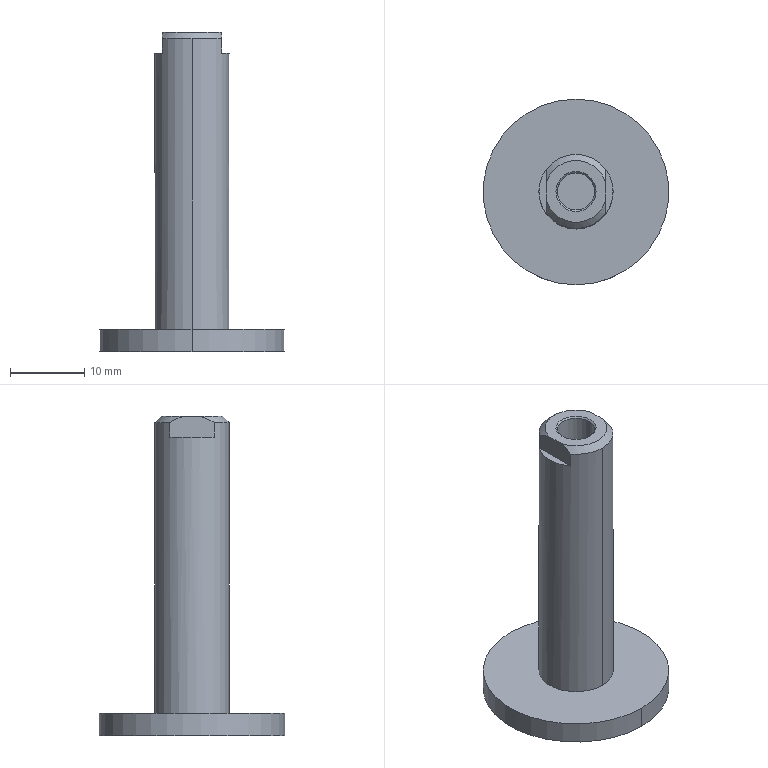Part | SolidWorks | features BaseBody 1 | 1 solid | 18 faces | box 25 x 25 x 43 mm | volume 4388 mm3 | plane 8 | cylinder 6 | cone 4 | commonest cylinder face diameters 5 x2 10 x2 25 x2
STEP:
#1=CARTESIAN_POINT('',(0.,-5.,-32.167));
#2=VERTEX_POINT('',#1);
#3=CARTESIAN_POINT('',(0.,5.,-32.167));
#4=VERTEX_POINT('',#3);
#5=CARTESIAN_POINT('',(0.,0.,-32.167));
#6=DIRECTION('',(0.,0.,1.));
#7=DIRECTION('',(0.,-1.,0.));
#8=AXIS2_PLACEMENT_3D('',#5,#6,#7);
#9=CIRCLE('',#8,5.);
#10=EDGE_CURVE('',#2,#4,#9,.T.);
#11=ORIENTED_EDGE('',*,*,#10,.T.);
#12=CARTESIAN_POINT('',(0.,5.,7.));
#13=VERTEX_POINT('',#12);
#14=CARTESIAN_POINT('',(0.,5.,1.833));
#15=DIRECTION('',(0.,0.,1.));
#16=VECTOR('',#15,1000.);
#17=LINE('',#14,#16);
#18=EDGE_CURVE('',#4,#13,#17,.T.);
#19=ORIENTED_EDGE('',*,*,#18,.T.);
#20=CARTESIAN_POINT('',(4.,3.,7.));
#21=VERTEX_POINT('',#20);
#22=CARTESIAN_POINT('',(0.,0.,7.));
#23=DIRECTION('',(0.,0.,-1.));
#24=DIRECTION('',(0.,-1.,0.));
#25=AXIS2_PLACEMENT_3D('',#22,#23,#24);
#26=CIRCLE('',#25,5.);
#27=EDGE_CURVE('',#13,#21,#26,.T.);
#28=ORIENTED_EDGE('',*,*,#27,.T.);
#29=CARTESIAN_POINT('',(4.,3.,5.033));
#30=VERTEX_POINT('',#29);
#31=CARTESIAN_POINT('',(4.,3.,1.833));
#32=DIRECTION('',(0.,0.,-1.));
#33=VECTOR('',#32,1000.);
#34=LINE('',#31,#33);
#35=EDGE_CURVE('',#21,#30,#34,.T.);
#36=ORIENTED_EDGE('',*,*,#35,.T.);
#37=CARTESIAN_POINT('',(4.,-3.,5.033));
#38=VERTEX_POINT('',#37);
#39=CARTESIAN_POINT('',(0.,0.,5.033));
#40=DIRECTION('',(0.,0.,-1.));
#41=DIRECTION('',(0.,-1.,0.));
#42=AXIS2_PLACEMENT_3D('',#39,#40,#41);
#43=CIRCLE('',#42,5.);
#44=EDGE_CURVE('',#30,#38,#43,.T.);
#45=ORIENTED_EDGE('',*,*,#44,.T.);
#46=CARTESIAN_POINT('',(4.,-3.,7.));
#47=VERTEX_POINT('',#46);
#48=CARTESIAN_POINT('',(4.,-3.,1.833));
#49=DIRECTION('',(0.,0.,1.));
#50=VECTOR('',#49,1000.);
#51=LINE('',#48,#50);
#52=EDGE_CURVE('',#38,#47,#51,.T.);
#53=ORIENTED_EDGE('',*,*,#52,.T.);
#54=CARTESIAN_POINT('',(0.,-5.,7.));
#55=VERTEX_POINT('',#54);
#56=CARTESIAN_POINT('',(0.,0.,7.));
#57=DIRECTION('',(0.,0.,-1.));
#58=DIRECTION('',(0.,-1.,0.));
#59=AXIS2_PLACEMENT_3D('',#56,#57,#58);
#60=CIRCLE('',#59,5.);
#61=EDGE_CURVE('',#47,#55,#60,.T.);
#62=ORIENTED_EDGE('',*,*,#61,.T.);
#63=CARTESIAN_POINT('',(0.,-5.,1.833));
#64=DIRECTION('',(0.,0.,1.));
#65=VECTOR('',#64,1000.);
#66=LINE('',#63,#65);
#67=EDGE_CURVE('',#2,#55,#66,.T.);
#68=ORIENTED_EDGE('',*,*,#67,.F.);
#69=EDGE_LOOP('',(#11,#19,#28,#36,#45,#53,#62,#68));
#70=FACE_OUTER_BOUND('',#69,.T.);
#71=CARTESIAN_POINT('',(0.,0.,1.833));
#72=DIRECTION('',(0.,0.,1.));
#73=DIRECTION('',(0.,-1.,0.));
#74=AXIS2_PLACEMENT_3D('',#71,#72,#73);
#75=CYLINDRICAL_SURFACE('',#74,5.);
#76=ADVANCED_FACE('',(#70),#75,.T.);
#77=CARTESIAN_POINT('',(0.,-12.5,-35.167));
#78=VERTEX_POINT('',#77);
#79=CARTESIAN_POINT('',(0.,12.5,-35.167));
#80=VERTEX_POINT('',#79);
#81=CARTESIAN_POINT('',(0.,0.,-35.167));
#82=DIRECTION('',(0.,0.,1.));
#83=DIRECTION('',(0.,-1.,0.));
#84=AXIS2_PLACEMENT_3D('',#81,#82,#83);
#85=CIRCLE('',#84,12.5);
#86=EDGE_CURVE('',#78,#80,#85,.T.);
#87=ORIENTED_EDGE('',*,*,#86,.T.);
#88=CARTESIAN_POINT('',(0.,12.5,-32.167));
#89=VERTEX_POINT('',#88);
#90=CARTESIAN_POINT('',(0.,12.5,1.833));
#91=DIRECTION('',(0.,0.,1.));
#92=VECTOR('',#91,1000.);
#93=LINE('',#90,#92);
#94=EDGE_CURVE('',#80,#89,#93,.T.);
#95=ORIENTED_EDGE('',*,*,#94,.T.);
#96=CARTESIAN_POINT('',(0.,-12.5,-32.167));
#97=VERTEX_POINT('',#96);
#98=CARTESIAN_POINT('',(0.,0.,-32.167));
#99=DIRECTION('',(0.,0.,-1.));
#100=DIRECTION('',(0.,-1.,0.));
#101=AXIS2_PLACEMENT_3D('',#98,#99,#100);
#102=CIRCLE('',#101,12.5);
#103=EDGE_CURVE('',#89,#97,#102,.T.);
#104=ORIENTED_EDGE('',*,*,#103,.T.);
#105=CARTESIAN_POINT('',(0.,-12.5,1.833));
#106=DIRECTION('',(0.,0.,1.));
#107=VECTOR('',#106,1000.);
#108=LINE('',#105,#107);
#109=EDGE_CURVE('',#78,#97,#108,.T.);
#110=ORIENTED_EDGE('',*,*,#109,.F.);
#111=EDGE_LOOP('',(#87,#95,#104,#110));
#112=FACE_OUTER_BOUND('',#111,.T.);
#113=CARTESIAN_POINT('',(0.,0.,1.833));
#114=DIRECTION('',(0.,0.,1.));
#115=DIRECTION('',(0.,-1.,0.));
#116=AXIS2_PLACEMENT_3D('',#113,#114,#115);
#117=CYLINDRICAL_SURFACE('',#116,12.5);
#118=ADVANCED_FACE('',(#112),#117,.T.);
#119=CARTESIAN_POINT('',(-2.5,0.,7.633));
#120=VERTEX_POINT('',#119);
#121=CARTESIAN_POINT('',(2.5,0.,7.633));
#122=VERTEX_POINT('',#121);
#123=CARTESIAN_POINT('',(0.,0.,7.633));
#124=DIRECTION('',(0.,0.,1.));
#125=DIRECTION('',(1.,0.,0.));
#126=AXIS2_PLACEMENT_3D('',#123,#124,#125);
#127=CIRCLE('',#126,2.5);
#128=EDGE_CURVE('',#120,#122,#127,.T.);
#129=ORIENTED_EDGE('',*,*,#128,.F.);
#130=CARTESIAN_POINT('',(-2.7,0.,7.833));
#131=VERTEX_POINT('',#130);
#132=CARTESIAN_POINT('',(-2.7,0.,7.833));
#133=DIRECTION('',(-0.7071,0.,0.7071));
#134=VECTOR('',#133,1000.);
#135=LINE('',#132,#134);
#136=EDGE_CURVE('',#120,#131,#135,.T.);
#137=ORIENTED_EDGE('',*,*,#136,.T.);
#138=CARTESIAN_POINT('',(2.7,0.,7.833));
#139=VERTEX_POINT('',#138);
#140=CARTESIAN_POINT('',(0.,0.,7.833));
#141=DIRECTION('',(0.,0.,1.));
#142=DIRECTION('',(1.,0.,0.));
#143=AXIS2_PLACEMENT_3D('',#140,#141,#142);
#144=CIRCLE('',#143,2.7);
#145=EDGE_CURVE('',#131,#139,#144,.T.);
#146=ORIENTED_EDGE('',*,*,#145,.T.);
#147=CARTESIAN_POINT('',(2.7,0.,7.833));
#148=DIRECTION('',(0.7071,0.,0.7071));
#149=VECTOR('',#148,1000.);
#150=LINE('',#147,#149);
#151=EDGE_CURVE('',#122,#139,#150,.T.);
#152=ORIENTED_EDGE('',*,*,#151,.F.);
#153=EDGE_LOOP('',(#129,#137,#146,#152));
#154=FACE_OUTER_BOUND('',#153,.T.);
#155=CARTESIAN_POINT('',(0.,0.,7.833));
#156=DIRECTION('',(0.,0.,1.));
#157=DIRECTION('',(1.,0.,0.));
#158=AXIS2_PLACEMENT_3D('',#155,#156,#157);
#159=CONICAL_SURFACE('',#158,2.7,0.7854);
#160=ADVANCED_FACE('',(#154),#159,.F.);
#161=CARTESIAN_POINT('',(-2.5,0.,-2.167));
#162=VERTEX_POINT('',#161);
#163=CARTESIAN_POINT('',(2.5,0.,-2.167));
#164=VERTEX_POINT('',#163);
#165=CARTESIAN_POINT('',(0.,0.,-2.167));
#166=DIRECTION('',(0.,0.,1.));
#167=DIRECTION('',(1.,0.,0.));
#168=AXIS2_PLACEMENT_3D('',#165,#166,#167);
#169=CIRCLE('',#168,2.5);
#170=EDGE_CURVE('',#162,#164,#169,.T.);
#171=ORIENTED_EDGE('',*,*,#170,.F.);
#172=CARTESIAN_POINT('',(-2.5,0.,-2.167));
#173=DIRECTION('',(0.,0.,1.));
#174=VECTOR('',#173,1000.);
#175=LINE('',#172,#174);
#176=EDGE_CURVE('',#162,#120,#175,.T.);
#177=ORIENTED_EDGE('',*,*,#176,.T.);
#178=ORIENTED_EDGE('',*,*,#128,.T.);
#179=CARTESIAN_POINT('',(2.5,0.,-2.167));
#180=DIRECTION('',(0.,0.,1.));
#181=VECTOR('',#180,1000.);
#182=LINE('',#179,#181);
#183=EDGE_CURVE('',#164,#122,#182,.T.);
#184=ORIENTED_EDGE('',*,*,#183,.F.);
#185=EDGE_LOOP('',(#171,#177,#178,#184));
#186=FACE_OUTER_BOUND('',#185,.T.);
#187=CARTESIAN_POINT('',(0.,0.,-2.167));
#188=DIRECTION('',(0.,0.,1.));
#189=DIRECTION('',(1.,0.,0.));
#190=AXIS2_PLACEMENT_3D('',#187,#188,#189);
#191=CYLINDRICAL_SURFACE('',#190,2.5);
#192=ADVANCED_FACE('',(#186),#191,.F.);
#193=ORIENTED_EDGE('',*,*,#18,.F.);
#194=CARTESIAN_POINT('',(0.,0.,-32.167));
#195=DIRECTION('',(0.,0.,1.));
#196=DIRECTION('',(0.,-1.,0.));
#197=AXIS2_PLACEMENT_3D('',#194,#195,#196);
#198=CIRCLE('',#197,5.);
#199=EDGE_CURVE('',#4,#2,#198,.T.);
#200=ORIENTED_EDGE('',*,*,#199,.T.);
#201=ORIENTED_EDGE('',*,*,#67,.T.);
#202=CARTESIAN_POINT('',(-4.,-3.,7.));
#203=VERTEX_POINT('',#202);
#204=CARTESIAN_POINT('',(0.,0.,7.));
#205=DIRECTION('',(0.,0.,-1.));
#206=DIRECTION('',(0.,-1.,0.));
#207=AXIS2_PLACEMENT_3D('',#204,#205,#206);
#208=CIRCLE('',#207,5.);
#209=EDGE_CURVE('',#55,#203,#208,.T.);
#210=ORIENTED_EDGE('',*,*,#209,.T.);
#211=CARTESIAN_POINT('',(-4.,-3.,5.033));
#212=VERTEX_POINT('',#211);
#213=CARTESIAN_POINT('',(-4.,-3.,1.833));
#214=DIRECTION('',(0.,0.,-1.));
#215=VECTOR('',#214,1000.);
#216=LINE('',#213,#215);
#217=EDGE_CURVE('',#203,#212,#216,.T.);
#218=ORIENTED_EDGE('',*,*,#217,.T.);
#219=CARTESIAN_POINT('',(-4.,3.,5.033));
#220=VERTEX_POINT('',#219);
#221=CARTESIAN_POINT('',(0.,0.,5.033));
#222=DIRECTION('',(0.,0.,-1.));
#223=DIRECTION('',(0.,-1.,0.));
#224=AXIS2_PLACEMENT_3D('',#221,#222,#223);
#225=CIRCLE('',#224,5.);
#226=EDGE_CURVE('',#212,#220,#225,.T.);
#227=ORIENTED_EDGE('',*,*,#226,.T.);
#228=CARTESIAN_POINT('',(-4.,3.,7.));
#229=VERTEX_POINT('',#228);
#230=CARTESIAN_POINT('',(-4.,3.,1.833));
#231=DIRECTION('',(0.,0.,1.));
#232=VECTOR('',#231,1000.);
#233=LINE('',#230,#232);
#234=EDGE_CURVE('',#220,#229,#233,.T.);
#235=ORIENTED_EDGE('',*,*,#234,.T.);
#236=CARTESIAN_POINT('',(0.,0.,7.));
#237=DIRECTION('',(0.,0.,-1.));
#238=DIRECTION('',(0.,-1.,0.));
#239=AXIS2_PLACEMENT_3D('',#236,#237,#238);
#240=CIRCLE('',#239,5.);
#241=EDGE_CURVE('',#229,#13,#240,.T.);
#242=ORIENTED_EDGE('',*,*,#241,.T.);
#243=EDGE_LOOP('',(#193,#200,#201,#210,#218,#227,#235,#242));
#244=FACE_OUTER_BOUND('',#243,.T.);
#245=CARTESIAN_POINT('',(0.,0.,1.833));
#246=DIRECTION('',(0.,0.,1.));
#247=DIRECTION('',(0.,-1.,0.));
#248=AXIS2_PLACEMENT_3D('',#245,#246,#247);
#249=CYLINDRICAL_SURFACE('',#248,5.);
#250=ADVANCED_FACE('',(#244),#249,.T.);
#251=ORIENTED_EDGE('',*,*,#61,.F.);
#252=CARTESIAN_POINT('',(4.,-1.167,7.833));
#253=VERTEX_POINT('',#252);
#254=CARTESIAN_POINT('',(4.,-3.,7.));
#255=CARTESIAN_POINT('',(4.,-2.71,7.174));
#256=CARTESIAN_POINT('',(4.,-2.415,7.335));
#257=CARTESIAN_POINT('',(4.,-1.807,7.619));
#258=CARTESIAN_POINT('',(4.,-1.494,7.742));
#259=CARTESIAN_POINT('',(4.,-1.167,7.833));
#260=B_SPLINE_CURVE_WITH_KNOTS('',3,(#254,#255,#256,#257,#258,#259),.UNSPECIFIED.,.F.,.F.,(4,2,4),(0.,0.001007,0.002014),.UNSPECIFIED.);
#261=EDGE_CURVE('',#47,#253,#260,.T.);
#262=ORIENTED_EDGE('',*,*,#261,.T.);
#263=CARTESIAN_POINT('',(-4.,-1.167,7.833));
#264=VERTEX_POINT('',#263);
#265=CARTESIAN_POINT('',(0.,0.,7.833));
#266=DIRECTION('',(0.,0.,-1.));
#267=DIRECTION('',(-1.,0.,0.));
#268=AXIS2_PLACEMENT_3D('',#265,#266,#267);
#269=CIRCLE('',#268,4.167);
#270=EDGE_CURVE('',#253,#264,#269,.T.);
#271=ORIENTED_EDGE('',*,*,#270,.T.);
#272=CARTESIAN_POINT('',(-4.,-1.167,7.833));
#273=CARTESIAN_POINT('',(-4.,-1.494,7.742));
#274=CARTESIAN_POINT('',(-4.,-1.807,7.619));
#275=CARTESIAN_POINT('',(-4.,-2.415,7.335));
#276=CARTESIAN_POINT('',(-4.,-2.71,7.174));
#277=CARTESIAN_POINT('',(-4.,-3.,7.));
#278=B_SPLINE_CURVE_WITH_KNOTS('',3,(#272,#273,#274,#275,#276,#277),.UNSPECIFIED.,.F.,.F.,(4,2,4),(0.,0.001007,0.002014),.UNSPECIFIED.);
#279=EDGE_CURVE('',#264,#203,#278,.T.);
#280=ORIENTED_EDGE('',*,*,#279,.T.);
#281=ORIENTED_EDGE('',*,*,#209,.F.);
#282=EDGE_LOOP('',(#251,#262,#271,#280,#281));
#283=FACE_OUTER_BOUND('',#282,.T.);
#284=CARTESIAN_POINT('',(0.,0.,7.));
#285=DIRECTION('',(0.,0.,-1.));
#286=DIRECTION('',(-1.,0.,0.));
#287=AXIS2_PLACEMENT_3D('',#284,#285,#286);
#288=CONICAL_SURFACE('',#287,5.,0.7854);
#289=ADVANCED_FACE('',(#283),#288,.T.);
#290=CARTESIAN_POINT('',(4.,5.5,5.033));
#291=DIRECTION('',(0.,-1.,0.));
#292=VECTOR('',#291,1000.);
#293=LINE('',#290,#292);
#294=EDGE_CURVE('',#30,#38,#293,.T.);
#295=ORIENTED_EDGE('',*,*,#294,.F.);
#296=ORIENTED_EDGE('',*,*,#35,.F.);
#297=CARTESIAN_POINT('',(4.,1.167,7.833));
#298=VERTEX_POINT('',#297);
#299=CARTESIAN_POINT('',(4.,1.167,7.833));
#300=CARTESIAN_POINT('',(4.,1.494,7.742));
#301=CARTESIAN_POINT('',(4.,1.807,7.619));
#302=CARTESIAN_POINT('',(4.,2.415,7.335));
#303=CARTESIAN_POINT('',(4.,2.71,7.174));
#304=CARTESIAN_POINT('',(4.,3.,7.));
#305=B_SPLINE_CURVE_WITH_KNOTS('',3,(#299,#300,#301,#302,#303,#304),.UNSPECIFIED.,.F.,.F.,(4,2,4),(0.,0.001007,0.002014),.UNSPECIFIED.);
#306=EDGE_CURVE('',#298,#21,#305,.T.);
#307=ORIENTED_EDGE('',*,*,#306,.F.);
#308=CARTESIAN_POINT('',(4.,5.5,7.833));
#309=DIRECTION('',(0.,1.,0.));
#310=VECTOR('',#309,1000.);
#311=LINE('',#308,#310);
#312=EDGE_CURVE('',#253,#298,#311,.T.);
#313=ORIENTED_EDGE('',*,*,#312,.F.);
#314=ORIENTED_EDGE('',*,*,#261,.F.);
#315=ORIENTED_EDGE('',*,*,#52,.F.);
#316=EDGE_LOOP('',(#295,#296,#307,#313,#314,#315));
#317=FACE_OUTER_BOUND('',#316,.T.);
#318=CARTESIAN_POINT('',(4.,5.5,5.033));
#319=DIRECTION('',(-1.,0.,0.));
#320=DIRECTION('',(0.,0.,1.));
#321=AXIS2_PLACEMENT_3D('',#318,#319,#320);
#322=PLANE('',#321);
#323=ADVANCED_FACE('',(#317),#322,.F.);
#324=ORIENTED_EDGE('',*,*,#44,.F.);
#325=ORIENTED_EDGE('',*,*,#294,.T.);
#326=EDGE_LOOP('',(#324,#325));
#327=FACE_OUTER_BOUND('',#326,.T.);
#328=CARTESIAN_POINT('',(4.,5.5,5.033));
#329=DIRECTION('',(0.,0.,1.));
#330=DIRECTION('',(1.,0.,0.));
#331=AXIS2_PLACEMENT_3D('',#328,#329,#330);
#332=PLANE('',#331);
#333=ADVANCED_FACE('',(#327),#332,.T.);
#334=ORIENTED_EDGE('',*,*,#306,.T.);
#335=ORIENTED_EDGE('',*,*,#27,.F.);
#336=ORIENTED_EDGE('',*,*,#241,.F.);
#337=CARTESIAN_POINT('',(-4.,1.167,7.833));
#338=VERTEX_POINT('',#337);
#339=CARTESIAN_POINT('',(-4.,3.,7.));
#340=CARTESIAN_POINT('',(-4.,2.71,7.174));
#341=CARTESIAN_POINT('',(-4.,2.415,7.335));
#342=CARTESIAN_POINT('',(-4.,1.807,7.619));
#343=CARTESIAN_POINT('',(-4.,1.494,7.742));
#344=CARTESIAN_POINT('',(-4.,1.167,7.833));
#345=B_SPLINE_CURVE_WITH_KNOTS('',3,(#339,#340,#341,#342,#343,#344),.UNSPECIFIED.,.F.,.F.,(4,2,4),(0.,0.001007,0.002014),.UNSPECIFIED.);
#346=EDGE_CURVE('',#229,#338,#345,.T.);
#347=ORIENTED_EDGE('',*,*,#346,.T.);
#348=CARTESIAN_POINT('',(0.,0.,7.833));
#349=DIRECTION('',(0.,0.,-1.));
#350=DIRECTION('',(-1.,0.,0.));
#351=AXIS2_PLACEMENT_3D('',#348,#349,#350);
#352=CIRCLE('',#351,4.167);
#353=EDGE_CURVE('',#338,#298,#352,.T.);
#354=ORIENTED_EDGE('',*,*,#353,.T.);
#355=EDGE_LOOP('',(#334,#335,#336,#347,#354));
#356=FACE_OUTER_BOUND('',#355,.T.);
#357=CARTESIAN_POINT('',(0.,0.,7.));
#358=DIRECTION('',(0.,0.,-1.));
#359=DIRECTION('',(-1.,0.,0.));
#360=AXIS2_PLACEMENT_3D('',#357,#358,#359);
#361=CONICAL_SURFACE('',#360,5.,0.7854);
#362=ADVANCED_FACE('',(#356),#361,.T.);
#363=CARTESIAN_POINT('',(0.,0.,-32.167));
#364=DIRECTION('',(0.,0.,-1.));
#365=DIRECTION('',(0.,-1.,0.));
#366=AXIS2_PLACEMENT_3D('',#363,#364,#365);
#367=CIRCLE('',#366,12.5);
#368=EDGE_CURVE('',#97,#89,#367,.T.);
#369=ORIENTED_EDGE('',*,*,#368,.F.);
#370=ORIENTED_EDGE('',*,*,#103,.F.);
#371=EDGE_LOOP('',(#369,#370));
#372=FACE_OUTER_BOUND('',#371,.T.);
#373=ORIENTED_EDGE('',*,*,#10,.F.);
#374=ORIENTED_EDGE('',*,*,#199,.F.);
#375=EDGE_LOOP('',(#373,#374));
#376=FACE_BOUND('',#375,.T.);
#377=CARTESIAN_POINT('',(0.,12.5,-32.167));
#378=DIRECTION('',(0.,0.,-1.));
#379=DIRECTION('',(0.,1.,0.));
#380=AXIS2_PLACEMENT_3D('',#377,#378,#379);
#381=PLANE('',#380);
#382=ADVANCED_FACE('',(#372,#376),#381,.F.);
#383=CARTESIAN_POINT('',(-4.,5.5,5.033));
#384=DIRECTION('',(0.,1.,0.));
#385=VECTOR('',#384,1000.);
#386=LINE('',#383,#385);
#387=EDGE_CURVE('',#212,#220,#386,.T.);
#388=ORIENTED_EDGE('',*,*,#387,.F.);
#389=ORIENTED_EDGE('',*,*,#217,.F.);
#390=ORIENTED_EDGE('',*,*,#279,.F.);
#391=CARTESIAN_POINT('',(-4.,5.5,7.833));
#392=DIRECTION('',(0.,-1.,0.));
#393=VECTOR('',#392,1000.);
#394=LINE('',#391,#393);
#395=EDGE_CURVE('',#338,#264,#394,.T.);
#396=ORIENTED_EDGE('',*,*,#395,.F.);
#397=ORIENTED_EDGE('',*,*,#346,.F.);
#398=ORIENTED_EDGE('',*,*,#234,.F.);
#399=EDGE_LOOP('',(#388,#389,#390,#396,#397,#398));
#400=FACE_OUTER_BOUND('',#399,.T.);
#401=CARTESIAN_POINT('',(-4.,5.5,5.033));
#402=DIRECTION('',(1.,0.,0.));
#403=DIRECTION('',(0.,1.,0.));
#404=AXIS2_PLACEMENT_3D('',#401,#402,#403);
#405=PLANE('',#404);
#406=ADVANCED_FACE('',(#400),#405,.F.);
#407=ORIENTED_EDGE('',*,*,#226,.F.);
#408=ORIENTED_EDGE('',*,*,#387,.T.);
#409=EDGE_LOOP('',(#407,#408));
#410=FACE_OUTER_BOUND('',#409,.T.);
#411=CARTESIAN_POINT('',(-4.,-5.5,5.033));
#412=DIRECTION('',(0.,0.,-1.));
#413=DIRECTION('',(-1.,0.,0.));
#414=AXIS2_PLACEMENT_3D('',#411,#412,#413);
#415=PLANE('',#414);
#416=ADVANCED_FACE('',(#410),#415,.F.);
#417=ORIENTED_EDGE('',*,*,#353,.F.);
#418=ORIENTED_EDGE('',*,*,#395,.T.);
#419=ORIENTED_EDGE('',*,*,#270,.F.);
#420=ORIENTED_EDGE('',*,*,#312,.T.);
#421=EDGE_LOOP('',(#417,#418,#419,#420));
#422=FACE_OUTER_BOUND('',#421,.T.);
#423=CARTESIAN_POINT('',(0.,0.,7.833));
#424=DIRECTION('',(0.,0.,1.));
#425=DIRECTION('',(1.,0.,0.));
#426=AXIS2_PLACEMENT_3D('',#423,#424,#425);
#427=CIRCLE('',#426,2.7);
#428=EDGE_CURVE('',#139,#131,#427,.T.);
#429=ORIENTED_EDGE('',*,*,#428,.F.);
#430=ORIENTED_EDGE('',*,*,#145,.F.);
#431=EDGE_LOOP('',(#429,#430));
#432=FACE_BOUND('',#431,.T.);
#433=CARTESIAN_POINT('',(0.,0.,7.833));
#434=DIRECTION('',(0.,0.,-1.));
#435=DIRECTION('',(0.,1.,0.));
#436=AXIS2_PLACEMENT_3D('',#433,#434,#435);
#437=PLANE('',#436);
#438=ADVANCED_FACE('',(#422,#432),#437,.F.);
#439=ORIENTED_EDGE('',*,*,#94,.F.);
#440=CARTESIAN_POINT('',(0.,0.,-35.167));
#441=DIRECTION('',(0.,0.,1.));
#442=DIRECTION('',(0.,-1.,0.));
#443=AXIS2_PLACEMENT_3D('',#440,#441,#442);
#444=CIRCLE('',#443,12.5);
#445=EDGE_CURVE('',#80,#78,#444,.T.);
#446=ORIENTED_EDGE('',*,*,#445,.T.);
#447=ORIENTED_EDGE('',*,*,#109,.T.);
#448=ORIENTED_EDGE('',*,*,#368,.T.);
#449=EDGE_LOOP('',(#439,#446,#447,#448));
#450=FACE_OUTER_BOUND('',#449,.T.);
#451=CARTESIAN_POINT('',(0.,0.,1.833));
#452=DIRECTION('',(0.,0.,1.));
#453=DIRECTION('',(0.,-1.,0.));
#454=AXIS2_PLACEMENT_3D('',#451,#452,#453);
#455=CYLINDRICAL_SURFACE('',#454,12.5);
#456=ADVANCED_FACE('',(#450),#455,.T.);
#457=ORIENTED_EDGE('',*,*,#136,.F.);
#458=CARTESIAN_POINT('',(0.,0.,7.633));
#459=DIRECTION('',(0.,0.,1.));
#460=DIRECTION('',(1.,0.,0.));
#461=AXIS2_PLACEMENT_3D('',#458,#459,#460);
#462=CIRCLE('',#461,2.5);
#463=EDGE_CURVE('',#122,#120,#462,.T.);
#464=ORIENTED_EDGE('',*,*,#463,.F.);
#465=ORIENTED_EDGE('',*,*,#151,.T.);
#466=ORIENTED_EDGE('',*,*,#428,.T.);
#467=EDGE_LOOP('',(#457,#464,#465,#466));
#468=FACE_OUTER_BOUND('',#467,.T.);
#469=CARTESIAN_POINT('',(0.,0.,7.833));
#470=DIRECTION('',(0.,0.,1.));
#471=DIRECTION('',(1.,0.,0.));
#472=AXIS2_PLACEMENT_3D('',#469,#470,#471);
#473=CONICAL_SURFACE('',#472,2.7,0.7854);
#474=ADVANCED_FACE('',(#468),#473,.F.);
#475=ORIENTED_EDGE('',*,*,#86,.F.);
#476=ORIENTED_EDGE('',*,*,#445,.F.);
#477=EDGE_LOOP('',(#475,#476));
#478=FACE_OUTER_BOUND('',#477,.T.);
#479=CARTESIAN_POINT('',(0.,12.5,-35.167));
#480=DIRECTION('',(0.,0.,1.));
#481=DIRECTION('',(0.,-1.,0.));
#482=AXIS2_PLACEMENT_3D('',#479,#480,#481);
#483=PLANE('',#482);
#484=ADVANCED_FACE('',(#478),#483,.F.);
#485=ORIENTED_EDGE('',*,*,#176,.F.);
#486=CARTESIAN_POINT('',(0.,0.,-2.167));
#487=DIRECTION('',(0.,0.,1.));
#488=DIRECTION('',(1.,0.,0.));
#489=AXIS2_PLACEMENT_3D('',#486,#487,#488);
#490=CIRCLE('',#489,2.5);
#491=EDGE_CURVE('',#164,#162,#490,.T.);
#492=ORIENTED_EDGE('',*,*,#491,.F.);
#493=ORIENTED_EDGE('',*,*,#183,.T.);
#494=ORIENTED_EDGE('',*,*,#463,.T.);
#495=EDGE_LOOP('',(#485,#492,#493,#494));
#496=FACE_OUTER_BOUND('',#495,.T.);
#497=CARTESIAN_POINT('',(0.,0.,-2.167));
#498=DIRECTION('',(0.,0.,1.));
#499=DIRECTION('',(1.,0.,0.));
#500=AXIS2_PLACEMENT_3D('',#497,#498,#499);
#501=CYLINDRICAL_SURFACE('',#500,2.5);
#502=ADVANCED_FACE('',(#496),#501,.F.);
#503=ORIENTED_EDGE('',*,*,#491,.T.);
#504=ORIENTED_EDGE('',*,*,#170,.T.);
#505=EDGE_LOOP('',(#503,#504));
#506=FACE_OUTER_BOUND('',#505,.T.);
#507=CARTESIAN_POINT('',(0.,0.,-2.167));
#508=DIRECTION('',(0.,0.,1.));
#509=DIRECTION('',(1.,0.,0.));
#510=AXIS2_PLACEMENT_3D('',#507,#508,#509);
#511=PLANE('',#510);
#512=ADVANCED_FACE('',(#506),#511,.T.);
#513=CLOSED_SHELL('',(#76,#118,#160,#192,#250,#289,#323,#333,#362,#382,#406,#416,#438,#456,#474,#484,#502,#512));
#514=MANIFOLD_SOLID_BREP('',#513);
#515=CARTESIAN_POINT('',(0.,0.,0.));
#516=DIRECTION('',(0.,0.,1.));
#517=DIRECTION('',(1.,0.,0.));
#518=AXIS2_PLACEMENT_3D('',#515,#516,#517);
#519=(LENGTH_UNIT()NAMED_UNIT(*)SI_UNIT(.MILLI.,.METRE.));
#520=UNCERTAINTY_MEASURE_WITH_UNIT(LENGTH_MEASURE(0.00001),#519,'','');
#521=(NAMED_UNIT(*)PLANE_ANGLE_UNIT()SI_UNIT($,.RADIAN.));
#522=(NAMED_UNIT(*)SI_UNIT($,.STERADIAN.)SOLID_ANGLE_UNIT());
#523=(GEOMETRIC_REPRESENTATION_CONTEXT(3)GLOBAL_UNCERTAINTY_ASSIGNED_CONTEXT((#520))GLOBAL_UNIT_ASSIGNED_CONTEXT((#519,#521,#522))REPRESENTATION_CONTEXT('',''));
#524=ADVANCED_BREP_SHAPE_REPRESENTATION('',(#514,#518),#523);